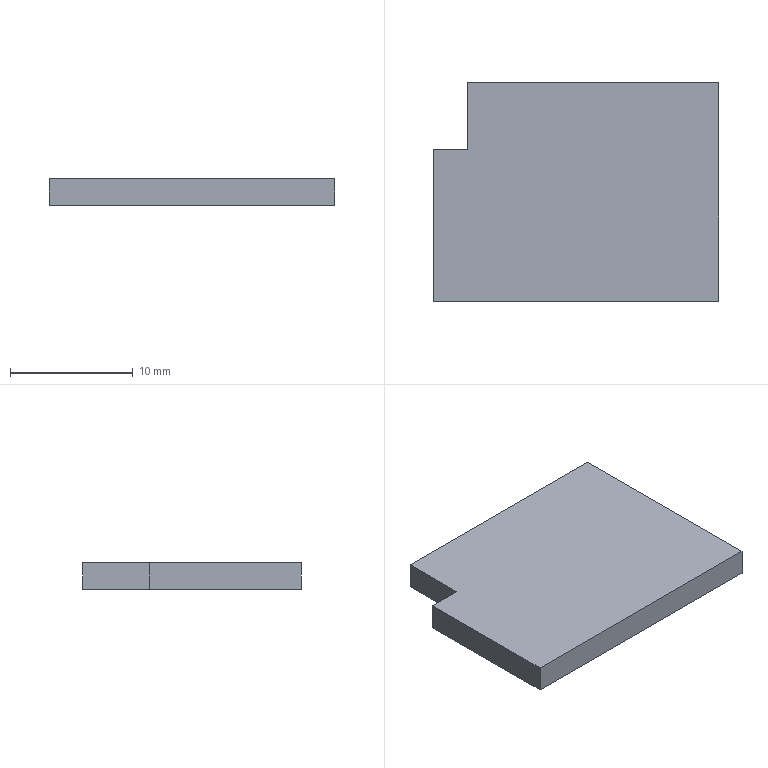Part | STEP file | RJ-USIO-V1_2-220411_203 | 1 solid | 8 faces | box 23.3 x 17.8 x 2.2 mm | volume 879.164 mm3 | plane 8
STEP:
#1=CARTESIAN_POINT('',(0.,0.,0.));
#2=DIRECTION('',(0.,0.,1.));
#3=DIRECTION('',(1.,0.,0.));
#4=AXIS2_PLACEMENT_3D('',#1,#2,#3);
#5=CARTESIAN_POINT('',(26.5,59.4,3.2));
#6=VERTEX_POINT('',#5);
#7=CARTESIAN_POINT('',(26.5,41.6,3.2));
#8=VERTEX_POINT('',#7);
#9=CARTESIAN_POINT('',(26.5,59.4,3.2));
#10=DIRECTION('',(0.000000044,-1.,0.));
#11=VECTOR('',#10,1.);
#12=LINE('',#9,#11);
#13=CARTESIAN_POINT('',(26.5,41.6,3.2));
#14=DIRECTION('',(0.,0.,-1.));
#15=DIRECTION('',(-0.000000044,1.,0.));
#16=AXIS2_PLACEMENT_3D('',#13,#14,#15);
#17=PLANE('',#16);
#18=CARTESIAN_POINT('',(17.8,0.));
#19=DIRECTION('',(-1.,0.));
#20=VECTOR('',#19,1.);
#21=LINE('',#18,#20);
#22=(GEOMETRIC_REPRESENTATION_CONTEXT(2)PARAMETRIC_REPRESENTATION_CONTEXT()REPRESENTATION_CONTEXT('',''));
#23=DEFINITIONAL_REPRESENTATION('',(#21),#22);
#24=PCURVE('',#17,#23);
#25=CARTESIAN_POINT('',(26.5,41.6,1.));
#26=DIRECTION('',(-1.,-0.000000044,0.));
#27=DIRECTION('',(0.000000044,-1.,0.));
#28=AXIS2_PLACEMENT_3D('',#25,#26,#27);
#29=PLANE('',#28);
#30=CARTESIAN_POINT('',(-17.8,2.2));
#31=DIRECTION('',(1.,0.));
#32=VECTOR('',#31,1.);
#33=LINE('',#30,#32);
#34=(GEOMETRIC_REPRESENTATION_CONTEXT(2)PARAMETRIC_REPRESENTATION_CONTEXT()REPRESENTATION_CONTEXT('',''));
#35=DEFINITIONAL_REPRESENTATION('',(#33),#34);
#36=PCURVE('',#29,#35);
#37=SURFACE_CURVE('',#12,(#24,#36),.PCURVE_S1.);
#38=EDGE_CURVE('',#6,#8,#37,.T.);
#39=ORIENTED_EDGE('',*,*,#38,.T.);
#40=CARTESIAN_POINT('',(3.2,41.6,3.2));
#41=VERTEX_POINT('',#40);
#42=CARTESIAN_POINT('',(26.5,41.6,3.2));
#43=DIRECTION('',(-1.,-0.000000044,0.));
#44=VECTOR('',#43,1.);
#45=LINE('',#42,#44);
#46=CARTESIAN_POINT('',(0.,0.));
#47=DIRECTION('',(0.,-1.));
#48=VECTOR('',#47,1.);
#49=LINE('',#46,#48);
#50=(GEOMETRIC_REPRESENTATION_CONTEXT(2)PARAMETRIC_REPRESENTATION_CONTEXT()REPRESENTATION_CONTEXT('',''));
#51=DEFINITIONAL_REPRESENTATION('',(#49),#50);
#52=PCURVE('',#17,#51);
#53=CARTESIAN_POINT('',(3.2,41.6,1.));
#54=DIRECTION('',(-0.000000044,1.,0.));
#55=DIRECTION('',(-1.,-0.000000044,0.));
#56=AXIS2_PLACEMENT_3D('',#53,#54,#55);
#57=PLANE('',#56);
#58=CARTESIAN_POINT('',(-23.3,2.2));
#59=DIRECTION('',(1.,0.));
#60=VECTOR('',#59,1.);
#61=LINE('',#58,#60);
#62=(GEOMETRIC_REPRESENTATION_CONTEXT(2)PARAMETRIC_REPRESENTATION_CONTEXT()REPRESENTATION_CONTEXT('',''));
#63=DEFINITIONAL_REPRESENTATION('',(#61),#62);
#64=PCURVE('',#57,#63);
#65=SURFACE_CURVE('',#45,(#52,#64),.PCURVE_S1.);
#66=EDGE_CURVE('',#8,#41,#65,.T.);
#67=ORIENTED_EDGE('',*,*,#66,.T.);
#68=CARTESIAN_POINT('',(3.2,54.,3.2));
#69=VERTEX_POINT('',#68);
#70=CARTESIAN_POINT('',(3.2,41.6,3.2));
#71=DIRECTION('',(-0.000000044,1.,0.));
#72=VECTOR('',#71,1.);
#73=LINE('',#70,#72);
#74=CARTESIAN_POINT('',(0.,-23.3));
#75=DIRECTION('',(1.,0.));
#76=VECTOR('',#75,1.);
#77=LINE('',#74,#76);
#78=(GEOMETRIC_REPRESENTATION_CONTEXT(2)PARAMETRIC_REPRESENTATION_CONTEXT()REPRESENTATION_CONTEXT('',''));
#79=DEFINITIONAL_REPRESENTATION('',(#77),#78);
#80=PCURVE('',#17,#79);
#81=CARTESIAN_POINT('',(3.2,54.,1.));
#82=DIRECTION('',(1.,0.000000044,0.));
#83=DIRECTION('',(-0.000000044,1.,0.));
#84=AXIS2_PLACEMENT_3D('',#81,#82,#83);
#85=PLANE('',#84);
#86=CARTESIAN_POINT('',(-12.4,2.2));
#87=DIRECTION('',(1.,0.));
#88=VECTOR('',#87,1.);
#89=LINE('',#86,#88);
#90=(GEOMETRIC_REPRESENTATION_CONTEXT(2)PARAMETRIC_REPRESENTATION_CONTEXT()REPRESENTATION_CONTEXT('',''));
#91=DEFINITIONAL_REPRESENTATION('',(#89),#90);
#92=PCURVE('',#85,#91);
#93=SURFACE_CURVE('',#73,(#80,#92),.PCURVE_S1.);
#94=EDGE_CURVE('',#41,#69,#93,.T.);
#95=ORIENTED_EDGE('',*,*,#94,.T.);
#96=CARTESIAN_POINT('',(6.,54.,3.2));
#97=VERTEX_POINT('',#96);
#98=CARTESIAN_POINT('',(3.2,54.,3.2));
#99=DIRECTION('',(1.,0.000000044,0.));
#100=VECTOR('',#99,1.);
#101=LINE('',#98,#100);
#102=CARTESIAN_POINT('',(12.4,-23.3));
#103=DIRECTION('',(0.,1.));
#104=VECTOR('',#103,1.);
#105=LINE('',#102,#104);
#106=(GEOMETRIC_REPRESENTATION_CONTEXT(2)PARAMETRIC_REPRESENTATION_CONTEXT()REPRESENTATION_CONTEXT('',''));
#107=DEFINITIONAL_REPRESENTATION('',(#105),#106);
#108=PCURVE('',#17,#107);
#109=CARTESIAN_POINT('',(6.,54.,1.));
#110=DIRECTION('',(0.000000044,-1.,0.));
#111=DIRECTION('',(1.,0.000000044,0.));
#112=AXIS2_PLACEMENT_3D('',#109,#110,#111);
#113=PLANE('',#112);
#114=CARTESIAN_POINT('',(-2.8,2.2));
#115=DIRECTION('',(1.,0.));
#116=VECTOR('',#115,1.);
#117=LINE('',#114,#116);
#118=(GEOMETRIC_REPRESENTATION_CONTEXT(2)PARAMETRIC_REPRESENTATION_CONTEXT()REPRESENTATION_CONTEXT('',''));
#119=DEFINITIONAL_REPRESENTATION('',(#117),#118);
#120=PCURVE('',#113,#119);
#121=SURFACE_CURVE('',#101,(#108,#120),.PCURVE_S1.);
#122=EDGE_CURVE('',#69,#97,#121,.T.);
#123=ORIENTED_EDGE('',*,*,#122,.T.);
#124=CARTESIAN_POINT('',(6.,59.4,3.2));
#125=VERTEX_POINT('',#124);
#126=CARTESIAN_POINT('',(6.,54.,3.2));
#127=DIRECTION('',(-0.000000044,1.,0.));
#128=VECTOR('',#127,1.);
#129=LINE('',#126,#128);
#130=CARTESIAN_POINT('',(12.4,-20.5));
#131=DIRECTION('',(1.,0.));
#132=VECTOR('',#131,1.);
#133=LINE('',#130,#132);
#134=(GEOMETRIC_REPRESENTATION_CONTEXT(2)PARAMETRIC_REPRESENTATION_CONTEXT()REPRESENTATION_CONTEXT('',''));
#135=DEFINITIONAL_REPRESENTATION('',(#133),#134);
#136=PCURVE('',#17,#135);
#137=CARTESIAN_POINT('',(6.,59.4,1.));
#138=DIRECTION('',(1.,0.000000044,0.));
#139=DIRECTION('',(-0.000000044,1.,0.));
#140=AXIS2_PLACEMENT_3D('',#137,#138,#139);
#141=PLANE('',#140);
#142=CARTESIAN_POINT('',(-5.4,2.2));
#143=DIRECTION('',(1.,0.));
#144=VECTOR('',#143,1.);
#145=LINE('',#142,#144);
#146=(GEOMETRIC_REPRESENTATION_CONTEXT(2)PARAMETRIC_REPRESENTATION_CONTEXT()REPRESENTATION_CONTEXT('',''));
#147=DEFINITIONAL_REPRESENTATION('',(#145),#146);
#148=PCURVE('',#141,#147);
#149=SURFACE_CURVE('',#129,(#136,#148),.PCURVE_S1.);
#150=EDGE_CURVE('',#97,#125,#149,.T.);
#151=ORIENTED_EDGE('',*,*,#150,.T.);
#152=CARTESIAN_POINT('',(6.,59.4,3.2));
#153=DIRECTION('',(1.,0.000000044,0.));
#154=VECTOR('',#153,1.);
#155=LINE('',#152,#154);
#156=CARTESIAN_POINT('',(17.8,-20.5));
#157=DIRECTION('',(0.,1.));
#158=VECTOR('',#157,1.);
#159=LINE('',#156,#158);
#160=(GEOMETRIC_REPRESENTATION_CONTEXT(2)PARAMETRIC_REPRESENTATION_CONTEXT()REPRESENTATION_CONTEXT('',''));
#161=DEFINITIONAL_REPRESENTATION('',(#159),#160);
#162=PCURVE('',#17,#161);
#163=CARTESIAN_POINT('',(26.5,59.4,1.));
#164=DIRECTION('',(0.000000044,-1.,0.));
#165=DIRECTION('',(1.,0.000000044,0.));
#166=AXIS2_PLACEMENT_3D('',#163,#164,#165);
#167=PLANE('',#166);
#168=CARTESIAN_POINT('',(-20.5,2.2));
#169=DIRECTION('',(1.,0.));
#170=VECTOR('',#169,1.);
#171=LINE('',#168,#170);
#172=(GEOMETRIC_REPRESENTATION_CONTEXT(2)PARAMETRIC_REPRESENTATION_CONTEXT()REPRESENTATION_CONTEXT('',''));
#173=DEFINITIONAL_REPRESENTATION('',(#171),#172);
#174=PCURVE('',#167,#173);
#175=SURFACE_CURVE('',#155,(#162,#174),.PCURVE_S1.);
#176=EDGE_CURVE('',#125,#6,#175,.T.);
#177=ORIENTED_EDGE('',*,*,#176,.T.);
#178=EDGE_LOOP('',(#39,#67,#95,#123,#151,#177));
#179=FACE_BOUND('',#178,.F.);
#180=ADVANCED_FACE('',(#179),#17,.F.);
#181=CARTESIAN_POINT('',(26.5,59.4,1.));
#182=VERTEX_POINT('',#181);
#183=CARTESIAN_POINT('',(26.5,41.6,1.));
#184=VERTEX_POINT('',#183);
#185=CARTESIAN_POINT('',(26.5,59.4,1.));
#186=DIRECTION('',(0.000000044,-1.,0.));
#187=VECTOR('',#186,1.);
#188=LINE('',#185,#187);
#189=CARTESIAN_POINT('',(-17.8,0.));
#190=DIRECTION('',(1.,0.));
#191=VECTOR('',#190,1.);
#192=LINE('',#189,#191);
#193=(GEOMETRIC_REPRESENTATION_CONTEXT(2)PARAMETRIC_REPRESENTATION_CONTEXT()REPRESENTATION_CONTEXT('',''));
#194=DEFINITIONAL_REPRESENTATION('',(#192),#193);
#195=PCURVE('',#29,#194);
#196=CARTESIAN_POINT('',(26.5,41.6,1.));
#197=DIRECTION('',(0.,0.,-1.));
#198=DIRECTION('',(-0.000000044,1.,0.));
#199=AXIS2_PLACEMENT_3D('',#196,#197,#198);
#200=PLANE('',#199);
#201=CARTESIAN_POINT('',(17.8,0.));
#202=DIRECTION('',(-1.,0.));
#203=VECTOR('',#202,1.);
#204=LINE('',#201,#203);
#205=(GEOMETRIC_REPRESENTATION_CONTEXT(2)PARAMETRIC_REPRESENTATION_CONTEXT()REPRESENTATION_CONTEXT('',''));
#206=DEFINITIONAL_REPRESENTATION('',(#204),#205);
#207=PCURVE('',#200,#206);
#208=SURFACE_CURVE('',#188,(#195,#207),.PCURVE_S1.);
#209=EDGE_CURVE('',#182,#184,#208,.T.);
#210=ORIENTED_EDGE('',*,*,#209,.T.);
#211=CARTESIAN_POINT('',(26.5,41.6,3.2));
#212=DIRECTION('',(0.,0.,-1.));
#213=VECTOR('',#212,1.);
#214=LINE('',#211,#213);
#215=CARTESIAN_POINT('',(0.,2.2));
#216=DIRECTION('',(0.,-1.));
#217=VECTOR('',#216,1.);
#218=LINE('',#215,#217);
#219=(GEOMETRIC_REPRESENTATION_CONTEXT(2)PARAMETRIC_REPRESENTATION_CONTEXT()REPRESENTATION_CONTEXT('',''));
#220=DEFINITIONAL_REPRESENTATION('',(#218),#219);
#221=PCURVE('',#29,#220);
#222=CARTESIAN_POINT('',(-23.3,2.2));
#223=DIRECTION('',(0.,-1.));
#224=VECTOR('',#223,1.);
#225=LINE('',#222,#224);
#226=(GEOMETRIC_REPRESENTATION_CONTEXT(2)PARAMETRIC_REPRESENTATION_CONTEXT()REPRESENTATION_CONTEXT('',''));
#227=DEFINITIONAL_REPRESENTATION('',(#225),#226);
#228=PCURVE('',#57,#227);
#229=SURFACE_CURVE('',#214,(#221,#228),.PCURVE_S1.);
#230=EDGE_CURVE('',#8,#184,#229,.T.);
#231=ORIENTED_EDGE('',*,*,#230,.F.);
#232=ORIENTED_EDGE('',*,*,#38,.F.);
#233=CARTESIAN_POINT('',(26.5,59.4,3.2));
#234=DIRECTION('',(0.,0.,-1.));
#235=VECTOR('',#234,1.);
#236=LINE('',#233,#235);
#237=CARTESIAN_POINT('',(-17.8,2.2));
#238=DIRECTION('',(0.,-1.));
#239=VECTOR('',#238,1.);
#240=LINE('',#237,#239);
#241=(GEOMETRIC_REPRESENTATION_CONTEXT(2)PARAMETRIC_REPRESENTATION_CONTEXT()REPRESENTATION_CONTEXT('',''));
#242=DEFINITIONAL_REPRESENTATION('',(#240),#241);
#243=PCURVE('',#29,#242);
#244=CARTESIAN_POINT('',(0.,2.2));
#245=DIRECTION('',(0.,-1.));
#246=VECTOR('',#245,1.);
#247=LINE('',#244,#246);
#248=(GEOMETRIC_REPRESENTATION_CONTEXT(2)PARAMETRIC_REPRESENTATION_CONTEXT()REPRESENTATION_CONTEXT('',''));
#249=DEFINITIONAL_REPRESENTATION('',(#247),#248);
#250=PCURVE('',#167,#249);
#251=SURFACE_CURVE('',#236,(#243,#250),.PCURVE_S1.);
#252=EDGE_CURVE('',#6,#182,#251,.T.);
#253=ORIENTED_EDGE('',*,*,#252,.T.);
#254=EDGE_LOOP('',(#210,#231,#232,#253));
#255=FACE_BOUND('',#254,.F.);
#256=ADVANCED_FACE('',(#255),#29,.F.);
#257=CARTESIAN_POINT('',(3.2,41.6,1.));
#258=VERTEX_POINT('',#257);
#259=CARTESIAN_POINT('',(26.5,41.6,1.));
#260=DIRECTION('',(-1.,-0.000000044,0.));
#261=VECTOR('',#260,1.);
#262=LINE('',#259,#261);
#263=CARTESIAN_POINT('',(0.,0.));
#264=DIRECTION('',(0.,-1.));
#265=VECTOR('',#264,1.);
#266=LINE('',#263,#265);
#267=(GEOMETRIC_REPRESENTATION_CONTEXT(2)PARAMETRIC_REPRESENTATION_CONTEXT()REPRESENTATION_CONTEXT('',''));
#268=DEFINITIONAL_REPRESENTATION('',(#266),#267);
#269=PCURVE('',#200,#268);
#270=CARTESIAN_POINT('',(-23.3,0.));
#271=DIRECTION('',(1.,0.));
#272=VECTOR('',#271,1.);
#273=LINE('',#270,#272);
#274=(GEOMETRIC_REPRESENTATION_CONTEXT(2)PARAMETRIC_REPRESENTATION_CONTEXT()REPRESENTATION_CONTEXT('',''));
#275=DEFINITIONAL_REPRESENTATION('',(#273),#274);
#276=PCURVE('',#57,#275);
#277=SURFACE_CURVE('',#262,(#269,#276),.PCURVE_S1.);
#278=EDGE_CURVE('',#184,#258,#277,.T.);
#279=ORIENTED_EDGE('',*,*,#278,.F.);
#280=ORIENTED_EDGE('',*,*,#209,.F.);
#281=CARTESIAN_POINT('',(6.,59.4,1.));
#282=VERTEX_POINT('',#281);
#283=CARTESIAN_POINT('',(6.,59.4,1.));
#284=DIRECTION('',(1.,0.000000044,0.));
#285=VECTOR('',#284,1.);
#286=LINE('',#283,#285);
#287=CARTESIAN_POINT('',(17.8,-20.5));
#288=DIRECTION('',(0.,1.));
#289=VECTOR('',#288,1.);
#290=LINE('',#287,#289);
#291=(GEOMETRIC_REPRESENTATION_CONTEXT(2)PARAMETRIC_REPRESENTATION_CONTEXT()REPRESENTATION_CONTEXT('',''));
#292=DEFINITIONAL_REPRESENTATION('',(#290),#291);
#293=PCURVE('',#200,#292);
#294=CARTESIAN_POINT('',(-20.5,0.));
#295=DIRECTION('',(1.,0.));
#296=VECTOR('',#295,1.);
#297=LINE('',#294,#296);
#298=(GEOMETRIC_REPRESENTATION_CONTEXT(2)PARAMETRIC_REPRESENTATION_CONTEXT()REPRESENTATION_CONTEXT('',''));
#299=DEFINITIONAL_REPRESENTATION('',(#297),#298);
#300=PCURVE('',#167,#299);
#301=SURFACE_CURVE('',#286,(#293,#300),.PCURVE_S1.);
#302=EDGE_CURVE('',#282,#182,#301,.T.);
#303=ORIENTED_EDGE('',*,*,#302,.F.);
#304=CARTESIAN_POINT('',(6.,54.,1.));
#305=VERTEX_POINT('',#304);
#306=CARTESIAN_POINT('',(6.,54.,1.));
#307=DIRECTION('',(-0.000000044,1.,0.));
#308=VECTOR('',#307,1.);
#309=LINE('',#306,#308);
#310=CARTESIAN_POINT('',(12.4,-20.5));
#311=DIRECTION('',(1.,0.));
#312=VECTOR('',#311,1.);
#313=LINE('',#310,#312);
#314=(GEOMETRIC_REPRESENTATION_CONTEXT(2)PARAMETRIC_REPRESENTATION_CONTEXT()REPRESENTATION_CONTEXT('',''));
#315=DEFINITIONAL_REPRESENTATION('',(#313),#314);
#316=PCURVE('',#200,#315);
#317=CARTESIAN_POINT('',(-5.4,0.));
#318=DIRECTION('',(1.,0.));
#319=VECTOR('',#318,1.);
#320=LINE('',#317,#319);
#321=(GEOMETRIC_REPRESENTATION_CONTEXT(2)PARAMETRIC_REPRESENTATION_CONTEXT()REPRESENTATION_CONTEXT('',''));
#322=DEFINITIONAL_REPRESENTATION('',(#320),#321);
#323=PCURVE('',#141,#322);
#324=SURFACE_CURVE('',#309,(#316,#323),.PCURVE_S1.);
#325=EDGE_CURVE('',#305,#282,#324,.T.);
#326=ORIENTED_EDGE('',*,*,#325,.F.);
#327=CARTESIAN_POINT('',(3.2,54.,1.));
#328=VERTEX_POINT('',#327);
#329=CARTESIAN_POINT('',(3.2,54.,1.));
#330=DIRECTION('',(1.,0.000000044,0.));
#331=VECTOR('',#330,1.);
#332=LINE('',#329,#331);
#333=CARTESIAN_POINT('',(12.4,-23.3));
#334=DIRECTION('',(0.,1.));
#335=VECTOR('',#334,1.);
#336=LINE('',#333,#335);
#337=(GEOMETRIC_REPRESENTATION_CONTEXT(2)PARAMETRIC_REPRESENTATION_CONTEXT()REPRESENTATION_CONTEXT('',''));
#338=DEFINITIONAL_REPRESENTATION('',(#336),#337);
#339=PCURVE('',#200,#338);
#340=CARTESIAN_POINT('',(-2.8,0.));
#341=DIRECTION('',(1.,0.));
#342=VECTOR('',#341,1.);
#343=LINE('',#340,#342);
#344=(GEOMETRIC_REPRESENTATION_CONTEXT(2)PARAMETRIC_REPRESENTATION_CONTEXT()REPRESENTATION_CONTEXT('',''));
#345=DEFINITIONAL_REPRESENTATION('',(#343),#344);
#346=PCURVE('',#113,#345);
#347=SURFACE_CURVE('',#332,(#339,#346),.PCURVE_S1.);
#348=EDGE_CURVE('',#328,#305,#347,.T.);
#349=ORIENTED_EDGE('',*,*,#348,.F.);
#350=CARTESIAN_POINT('',(3.2,41.6,1.));
#351=DIRECTION('',(-0.000000044,1.,0.));
#352=VECTOR('',#351,1.);
#353=LINE('',#350,#352);
#354=CARTESIAN_POINT('',(0.,-23.3));
#355=DIRECTION('',(1.,0.));
#356=VECTOR('',#355,1.);
#357=LINE('',#354,#356);
#358=(GEOMETRIC_REPRESENTATION_CONTEXT(2)PARAMETRIC_REPRESENTATION_CONTEXT()REPRESENTATION_CONTEXT('',''));
#359=DEFINITIONAL_REPRESENTATION('',(#357),#358);
#360=PCURVE('',#200,#359);
#361=CARTESIAN_POINT('',(-12.4,0.));
#362=DIRECTION('',(1.,0.));
#363=VECTOR('',#362,1.);
#364=LINE('',#361,#363);
#365=(GEOMETRIC_REPRESENTATION_CONTEXT(2)PARAMETRIC_REPRESENTATION_CONTEXT()REPRESENTATION_CONTEXT('',''));
#366=DEFINITIONAL_REPRESENTATION('',(#364),#365);
#367=PCURVE('',#85,#366);
#368=SURFACE_CURVE('',#353,(#360,#367),.PCURVE_S1.);
#369=EDGE_CURVE('',#258,#328,#368,.T.);
#370=ORIENTED_EDGE('',*,*,#369,.F.);
#371=EDGE_LOOP('',(#279,#280,#303,#326,#349,#370));
#372=FACE_BOUND('',#371,.F.);
#373=ADVANCED_FACE('',(#372),#200,.T.);
#374=ORIENTED_EDGE('',*,*,#278,.T.);
#375=CARTESIAN_POINT('',(3.2,41.6,3.2));
#376=DIRECTION('',(0.,0.,-1.));
#377=VECTOR('',#376,1.);
#378=LINE('',#375,#377);
#379=CARTESIAN_POINT('',(0.,2.2));
#380=DIRECTION('',(0.,-1.));
#381=VECTOR('',#380,1.);
#382=LINE('',#379,#381);
#383=(GEOMETRIC_REPRESENTATION_CONTEXT(2)PARAMETRIC_REPRESENTATION_CONTEXT()REPRESENTATION_CONTEXT('',''));
#384=DEFINITIONAL_REPRESENTATION('',(#382),#383);
#385=PCURVE('',#57,#384);
#386=CARTESIAN_POINT('',(-12.4,2.2));
#387=DIRECTION('',(0.,-1.));
#388=VECTOR('',#387,1.);
#389=LINE('',#386,#388);
#390=(GEOMETRIC_REPRESENTATION_CONTEXT(2)PARAMETRIC_REPRESENTATION_CONTEXT()REPRESENTATION_CONTEXT('',''));
#391=DEFINITIONAL_REPRESENTATION('',(#389),#390);
#392=PCURVE('',#85,#391);
#393=SURFACE_CURVE('',#378,(#385,#392),.PCURVE_S1.);
#394=EDGE_CURVE('',#41,#258,#393,.T.);
#395=ORIENTED_EDGE('',*,*,#394,.F.);
#396=ORIENTED_EDGE('',*,*,#66,.F.);
#397=ORIENTED_EDGE('',*,*,#230,.T.);
#398=EDGE_LOOP('',(#374,#395,#396,#397));
#399=FACE_BOUND('',#398,.F.);
#400=ADVANCED_FACE('',(#399),#57,.F.);
#401=ORIENTED_EDGE('',*,*,#369,.T.);
#402=CARTESIAN_POINT('',(3.2,54.,3.2));
#403=DIRECTION('',(0.,0.,-1.));
#404=VECTOR('',#403,1.);
#405=LINE('',#402,#404);
#406=CARTESIAN_POINT('',(0.,2.2));
#407=DIRECTION('',(0.,-1.));
#408=VECTOR('',#407,1.);
#409=LINE('',#406,#408);
#410=(GEOMETRIC_REPRESENTATION_CONTEXT(2)PARAMETRIC_REPRESENTATION_CONTEXT()REPRESENTATION_CONTEXT('',''));
#411=DEFINITIONAL_REPRESENTATION('',(#409),#410);
#412=PCURVE('',#85,#411);
#413=CARTESIAN_POINT('',(-2.8,2.2));
#414=DIRECTION('',(0.,-1.));
#415=VECTOR('',#414,1.);
#416=LINE('',#413,#415);
#417=(GEOMETRIC_REPRESENTATION_CONTEXT(2)PARAMETRIC_REPRESENTATION_CONTEXT()REPRESENTATION_CONTEXT('',''));
#418=DEFINITIONAL_REPRESENTATION('',(#416),#417);
#419=PCURVE('',#113,#418);
#420=SURFACE_CURVE('',#405,(#412,#419),.PCURVE_S1.);
#421=EDGE_CURVE('',#69,#328,#420,.T.);
#422=ORIENTED_EDGE('',*,*,#421,.F.);
#423=ORIENTED_EDGE('',*,*,#94,.F.);
#424=ORIENTED_EDGE('',*,*,#394,.T.);
#425=EDGE_LOOP('',(#401,#422,#423,#424));
#426=FACE_BOUND('',#425,.F.);
#427=ADVANCED_FACE('',(#426),#85,.F.);
#428=ORIENTED_EDGE('',*,*,#348,.T.);
#429=CARTESIAN_POINT('',(6.,54.,3.2));
#430=DIRECTION('',(0.,0.,-1.));
#431=VECTOR('',#430,1.);
#432=LINE('',#429,#431);
#433=CARTESIAN_POINT('',(0.,2.2));
#434=DIRECTION('',(0.,-1.));
#435=VECTOR('',#434,1.);
#436=LINE('',#433,#435);
#437=(GEOMETRIC_REPRESENTATION_CONTEXT(2)PARAMETRIC_REPRESENTATION_CONTEXT()REPRESENTATION_CONTEXT('',''));
#438=DEFINITIONAL_REPRESENTATION('',(#436),#437);
#439=PCURVE('',#113,#438);
#440=CARTESIAN_POINT('',(-5.4,2.2));
#441=DIRECTION('',(0.,-1.));
#442=VECTOR('',#441,1.);
#443=LINE('',#440,#442);
#444=(GEOMETRIC_REPRESENTATION_CONTEXT(2)PARAMETRIC_REPRESENTATION_CONTEXT()REPRESENTATION_CONTEXT('',''));
#445=DEFINITIONAL_REPRESENTATION('',(#443),#444);
#446=PCURVE('',#141,#445);
#447=SURFACE_CURVE('',#432,(#439,#446),.PCURVE_S1.);
#448=EDGE_CURVE('',#97,#305,#447,.T.);
#449=ORIENTED_EDGE('',*,*,#448,.F.);
#450=ORIENTED_EDGE('',*,*,#122,.F.);
#451=ORIENTED_EDGE('',*,*,#421,.T.);
#452=EDGE_LOOP('',(#428,#449,#450,#451));
#453=FACE_BOUND('',#452,.F.);
#454=ADVANCED_FACE('',(#453),#113,.F.);
#455=ORIENTED_EDGE('',*,*,#325,.T.);
#456=CARTESIAN_POINT('',(6.,59.4,3.2));
#457=DIRECTION('',(0.,0.,-1.));
#458=VECTOR('',#457,1.);
#459=LINE('',#456,#458);
#460=CARTESIAN_POINT('',(0.,2.2));
#461=DIRECTION('',(0.,-1.));
#462=VECTOR('',#461,1.);
#463=LINE('',#460,#462);
#464=(GEOMETRIC_REPRESENTATION_CONTEXT(2)PARAMETRIC_REPRESENTATION_CONTEXT()REPRESENTATION_CONTEXT('',''));
#465=DEFINITIONAL_REPRESENTATION('',(#463),#464);
#466=PCURVE('',#141,#465);
#467=CARTESIAN_POINT('',(-20.5,2.2));
#468=DIRECTION('',(0.,-1.));
#469=VECTOR('',#468,1.);
#470=LINE('',#467,#469);
#471=(GEOMETRIC_REPRESENTATION_CONTEXT(2)PARAMETRIC_REPRESENTATION_CONTEXT()REPRESENTATION_CONTEXT('',''));
#472=DEFINITIONAL_REPRESENTATION('',(#470),#471);
#473=PCURVE('',#167,#472);
#474=SURFACE_CURVE('',#459,(#466,#473),.PCURVE_S1.);
#475=EDGE_CURVE('',#125,#282,#474,.T.);
#476=ORIENTED_EDGE('',*,*,#475,.F.);
#477=ORIENTED_EDGE('',*,*,#150,.F.);
#478=ORIENTED_EDGE('',*,*,#448,.T.);
#479=EDGE_LOOP('',(#455,#476,#477,#478));
#480=FACE_BOUND('',#479,.F.);
#481=ADVANCED_FACE('',(#480),#141,.F.);
#482=ORIENTED_EDGE('',*,*,#302,.T.);
#483=ORIENTED_EDGE('',*,*,#252,.F.);
#484=ORIENTED_EDGE('',*,*,#176,.F.);
#485=ORIENTED_EDGE('',*,*,#475,.T.);
#486=EDGE_LOOP('',(#482,#483,#484,#485));
#487=FACE_BOUND('',#486,.F.);
#488=ADVANCED_FACE('',(#487),#167,.F.);
#489=CLOSED_SHELL('',(#180,#256,#373,#400,#427,#454,#481,#488));
#490=MANIFOLD_SOLID_BREP('',#489);
#491=(LENGTH_UNIT()NAMED_UNIT(*)SI_UNIT(.MILLI.,.METRE.));
#492=UNCERTAINTY_MEASURE_WITH_UNIT(LENGTH_MEASURE(0.0000001),#491,'','');
#493=(NAMED_UNIT(*)PLANE_ANGLE_UNIT()SI_UNIT($,.RADIAN.));
#494=(NAMED_UNIT(*)SI_UNIT($,.STERADIAN.)SOLID_ANGLE_UNIT());
#495=(GEOMETRIC_REPRESENTATION_CONTEXT(3)GLOBAL_UNCERTAINTY_ASSIGNED_CONTEXT((#492))GLOBAL_UNIT_ASSIGNED_CONTEXT((#491,#493,#494))REPRESENTATION_CONTEXT('',''));
#496=ADVANCED_BREP_SHAPE_REPRESENTATION('',(#4,#490),#495);